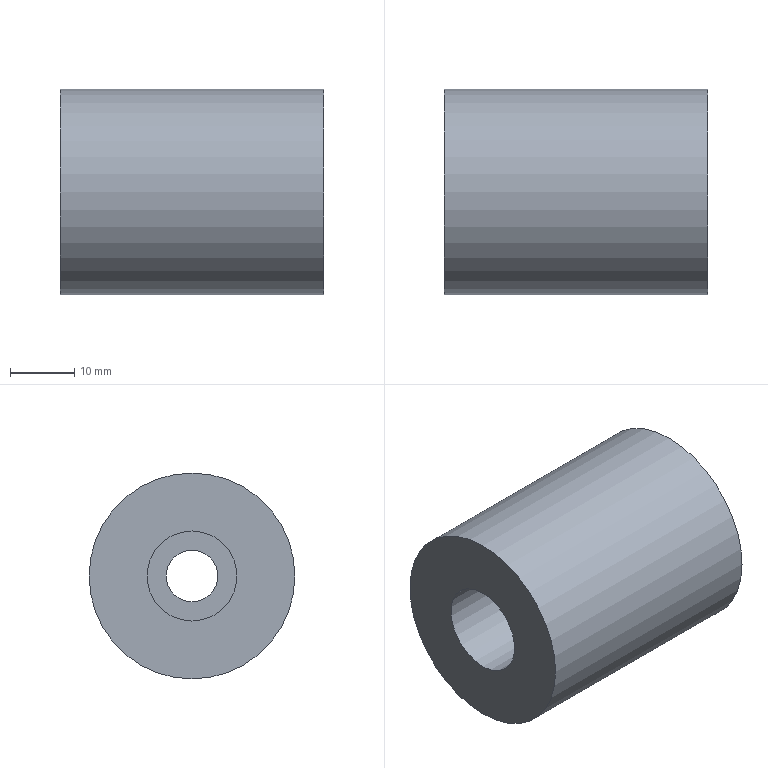Part | NX | 1 solid | 6 faces | box 41 x 32 x 32 mm | volume 28840 mm3 | cylinder 3 | plane 3 | commonest cylinder face diameters 8 x1 14 x1 32 x1
STEP:
#1=CARTESIAN_POINT('',(20.5,0.,-4.));
#2=VERTEX_POINT('',#1);
#3=CARTESIAN_POINT('',(20.5,0.,0.));
#4=DIRECTION('',(1.,0.,0.));
#5=DIRECTION('',(0.,0.,-1.));
#6=AXIS2_PLACEMENT_3D('',#3,#4,#5);
#7=CIRCLE('',#6,4.);
#8=EDGE_CURVE('',#2,#2,#7,.T.);
#9=ORIENTED_EDGE('',*,*,#8,.T.);
#10=EDGE_LOOP('',(#9));
#11=FACE_BOUND('',#10,.T.);
#12=CARTESIAN_POINT('',(-0.5,0.,4.));
#13=VERTEX_POINT('',#12);
#14=CARTESIAN_POINT('',(-0.5,0.,0.));
#15=DIRECTION('',(-1.,0.,0.));
#16=DIRECTION('',(0.,0.,1.));
#17=AXIS2_PLACEMENT_3D('',#14,#15,#16);
#18=CIRCLE('',#17,4.);
#19=EDGE_CURVE('',#13,#13,#18,.F.);
#20=ORIENTED_EDGE('',*,*,#19,.F.);
#21=EDGE_LOOP('',(#20));
#22=FACE_BOUND('',#21,.T.);
#23=CARTESIAN_POINT('',(-20.5,0.,0.));
#24=DIRECTION('',(1.,0.,0.));
#25=DIRECTION('',(0.,0.,-1.));
#26=AXIS2_PLACEMENT_3D('',#23,#24,#25);
#27=CYLINDRICAL_SURFACE('',#26,4.);
#28=ADVANCED_FACE('',(#11,#22),#27,.F.);
#29=CARTESIAN_POINT('',(20.5,0.,-16.));
#30=VERTEX_POINT('',#29);
#31=CARTESIAN_POINT('',(20.5,0.,0.));
#32=DIRECTION('',(1.,0.,0.));
#33=DIRECTION('',(0.,0.,-1.));
#34=AXIS2_PLACEMENT_3D('',#31,#32,#33);
#35=CIRCLE('',#34,16.);
#36=EDGE_CURVE('',#30,#30,#35,.T.);
#37=ORIENTED_EDGE('',*,*,#36,.F.);
#38=EDGE_LOOP('',(#37));
#39=FACE_BOUND('',#38,.T.);
#40=CARTESIAN_POINT('',(-20.5,0.,-16.));
#41=VERTEX_POINT('',#40);
#42=CARTESIAN_POINT('',(-20.5,0.,0.));
#43=DIRECTION('',(1.,0.,0.));
#44=DIRECTION('',(0.,0.,-1.));
#45=AXIS2_PLACEMENT_3D('',#42,#43,#44);
#46=CIRCLE('',#45,16.);
#47=EDGE_CURVE('',#41,#41,#46,.T.);
#48=ORIENTED_EDGE('',*,*,#47,.T.);
#49=EDGE_LOOP('',(#48));
#50=FACE_BOUND('',#49,.T.);
#51=CARTESIAN_POINT('',(20.5,0.,0.));
#52=DIRECTION('',(-1.,0.,0.));
#53=DIRECTION('',(0.,0.,1.));
#54=AXIS2_PLACEMENT_3D('',#51,#52,#53);
#55=CYLINDRICAL_SURFACE('',#54,16.);
#56=ADVANCED_FACE('',(#39,#50),#55,.T.);
#57=ORIENTED_EDGE('',*,*,#8,.F.);
#58=EDGE_LOOP('',(#57));
#59=FACE_BOUND('',#58,.T.);
#60=ORIENTED_EDGE('',*,*,#36,.T.);
#61=EDGE_LOOP('',(#60));
#62=FACE_BOUND('',#61,.T.);
#63=CARTESIAN_POINT('',(20.5,0.,0.));
#64=DIRECTION('',(1.,0.,0.));
#65=DIRECTION('',(0.,0.,-1.));
#66=AXIS2_PLACEMENT_3D('',#63,#64,#65);
#67=PLANE('',#66);
#68=ADVANCED_FACE('',(#59,#62),#67,.T.);
#69=CARTESIAN_POINT('',(-20.5,0.,7.));
#70=VERTEX_POINT('',#69);
#71=CARTESIAN_POINT('',(-20.5,0.,0.));
#72=DIRECTION('',(-1.,0.,0.));
#73=DIRECTION('',(0.,0.,1.));
#74=AXIS2_PLACEMENT_3D('',#71,#72,#73);
#75=CIRCLE('',#74,7.);
#76=EDGE_CURVE('',#70,#70,#75,.T.);
#77=ORIENTED_EDGE('',*,*,#76,.F.);
#78=EDGE_LOOP('',(#77));
#79=FACE_BOUND('',#78,.T.);
#80=ORIENTED_EDGE('',*,*,#47,.F.);
#81=EDGE_LOOP('',(#80));
#82=FACE_BOUND('',#81,.T.);
#83=CARTESIAN_POINT('',(-20.5,0.,0.));
#84=DIRECTION('',(1.,0.,0.));
#85=DIRECTION('',(0.,0.,-1.));
#86=AXIS2_PLACEMENT_3D('',#83,#84,#85);
#87=PLANE('',#86);
#88=ADVANCED_FACE('',(#79,#82),#87,.F.);
#89=CARTESIAN_POINT('',(-0.5,0.,7.));
#90=VERTEX_POINT('',#89);
#91=CARTESIAN_POINT('',(-0.5,0.,0.));
#92=DIRECTION('',(-1.,0.,0.));
#93=DIRECTION('',(0.,0.,1.));
#94=AXIS2_PLACEMENT_3D('',#91,#92,#93);
#95=CIRCLE('',#94,7.);
#96=EDGE_CURVE('',#90,#90,#95,.T.);
#97=ORIENTED_EDGE('',*,*,#96,.T.);
#98=EDGE_LOOP('',(#97));
#99=FACE_BOUND('',#98,.T.);
#100=ORIENTED_EDGE('',*,*,#19,.T.);
#101=EDGE_LOOP('',(#100));
#102=FACE_BOUND('',#101,.T.);
#103=CARTESIAN_POINT('',(-0.5,0.,0.));
#104=DIRECTION('',(-1.,0.,0.));
#105=DIRECTION('',(0.,0.,1.));
#106=AXIS2_PLACEMENT_3D('',#103,#104,#105);
#107=PLANE('',#106);
#108=ADVANCED_FACE('',(#99,#102),#107,.T.);
#109=ORIENTED_EDGE('',*,*,#96,.F.);
#110=EDGE_LOOP('',(#109));
#111=FACE_BOUND('',#110,.T.);
#112=ORIENTED_EDGE('',*,*,#76,.T.);
#113=EDGE_LOOP('',(#112));
#114=FACE_BOUND('',#113,.T.);
#115=CARTESIAN_POINT('',(-0.5,0.,0.));
#116=DIRECTION('',(-1.,0.,0.));
#117=DIRECTION('',(0.,0.,1.));
#118=AXIS2_PLACEMENT_3D('',#115,#116,#117);
#119=CYLINDRICAL_SURFACE('',#118,7.);
#120=ADVANCED_FACE('',(#111,#114),#119,.F.);
#121=CLOSED_SHELL('',(#28,#56,#68,#88,#108,#120));
#122=MANIFOLD_SOLID_BREP('',#121);
#123=(LENGTH_UNIT()NAMED_UNIT(*)SI_UNIT(.MILLI.,.METRE.));
#124=UNCERTAINTY_MEASURE_WITH_UNIT(LENGTH_MEASURE(0.00001),#123,'','');
#125=(NAMED_UNIT(*)PLANE_ANGLE_UNIT()SI_UNIT($,.RADIAN.));
#126=(NAMED_UNIT(*)SI_UNIT($,.STERADIAN.)SOLID_ANGLE_UNIT());
#127=(GEOMETRIC_REPRESENTATION_CONTEXT(3)GLOBAL_UNCERTAINTY_ASSIGNED_CONTEXT((#124))GLOBAL_UNIT_ASSIGNED_CONTEXT((#123,#125,#126))REPRESENTATION_CONTEXT('',''));
#128=ADVANCED_BREP_SHAPE_REPRESENTATION('',(#122),#127);